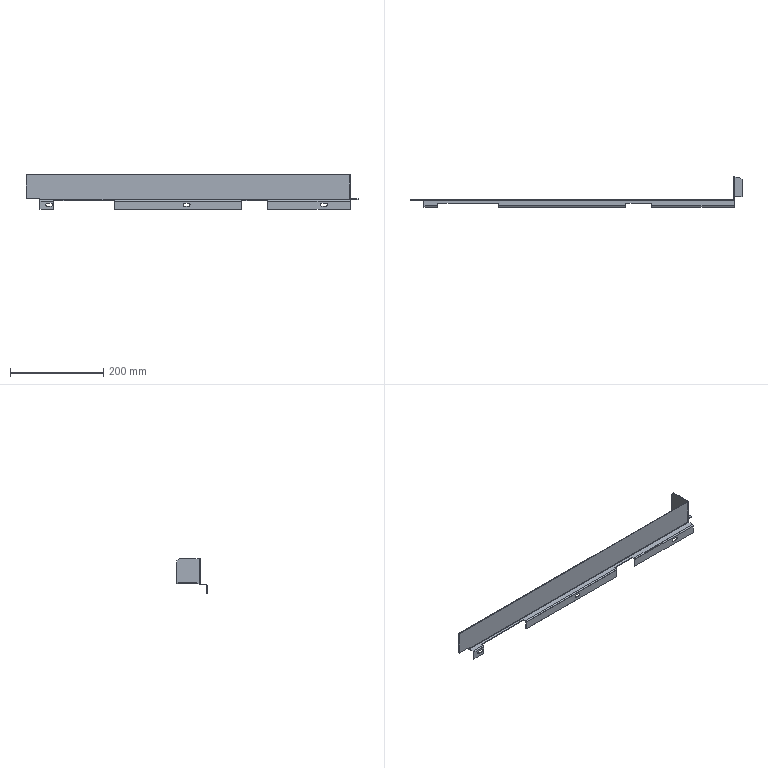Part | STEP file | 1 solid | 79 faces | box 713.5 x 64.5 x 74.5 mm | volume 87062 mm3 | plane 61 | cylinder 18 | commonest cylinder face diameters 2 x6 5 x6 7 x6